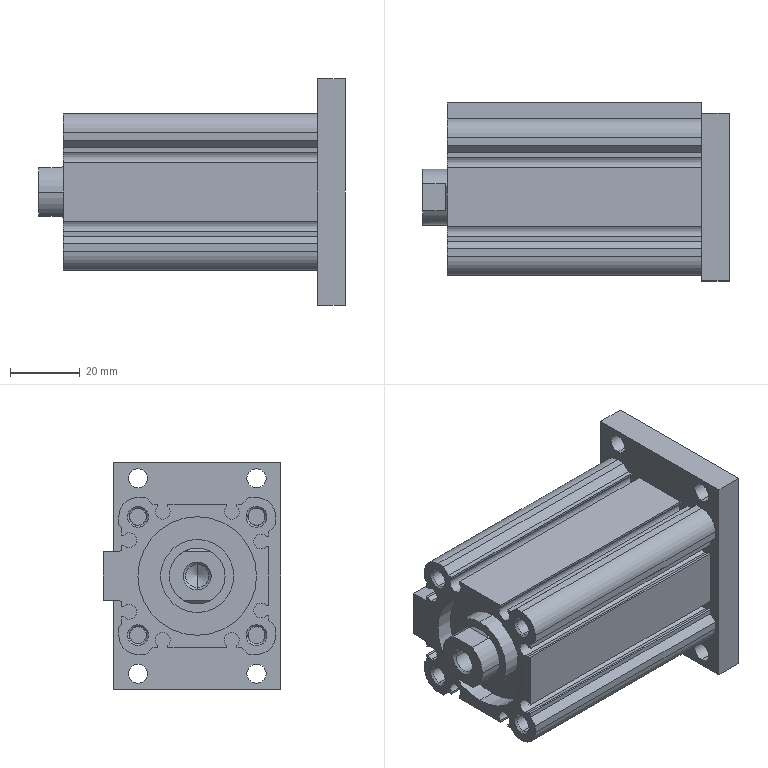Part | STEP file | CQ2G32-50DZ_0_0_0_ | 3 solids | 242 faces | box 88 x 51 x 65 mm | volume 108830 mm3 | cylinder 108 | plane 94 | cone 40 | commonest cylinder face diameters 4.26 x18 4.917 x16 6 x16 11 x12 5.5 x8 6.6 x8